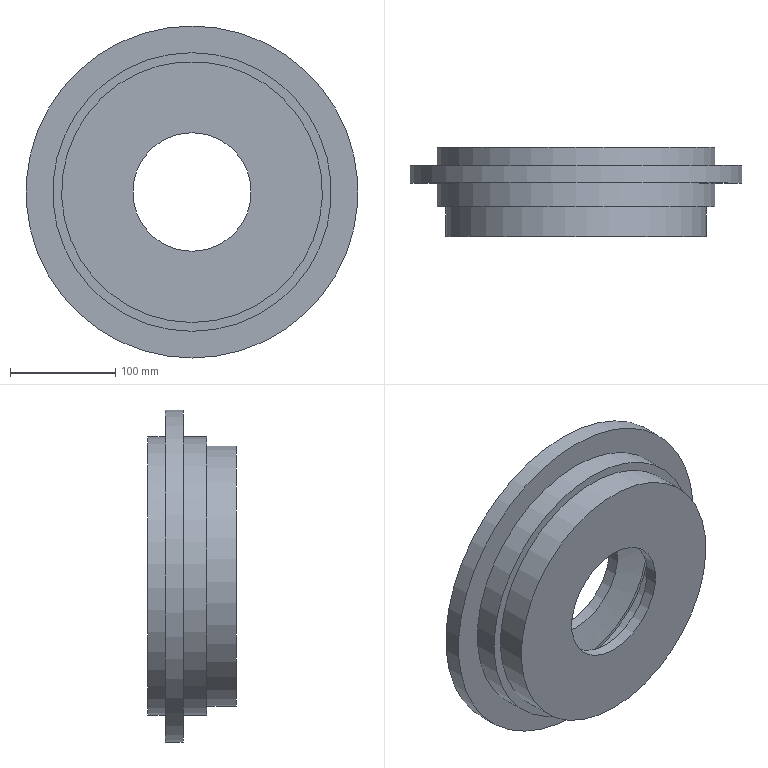Part | NX | features SIMPLE HOLE 4, CHAMFER 3, DATUM_CSYS 1, Delete Body 1, LINKED_BODY 1, SCALE 1, SKETCH 1, SWP104 1 | 1 solid | 18 faces | box 315 x 84.375 x 315 mm | volume 2887099 mm3 | plane 8 | cylinder 8 | cone 2 | commonest cylinder face diameters 112.5 x2 264.375 x2 185.625 x1 208.125 x1 247.5 x1 315 x1
STEP:
#1=CARTESIAN_POINT('',(-2029.479,-199.375,-310.332));
#2=VERTEX_POINT('',#1);
#3=CARTESIAN_POINT('',(-2029.479,-199.375,-366.582));
#4=DIRECTION('',(0.,1.,0.));
#5=DIRECTION('',(0.,0.,1.));
#6=AXIS2_PLACEMENT_3D('',#3,#4,#5);
#7=CIRCLE('',#6,56.25);
#8=EDGE_CURVE('',#2,#2,#7,.T.);
#9=ORIENTED_EDGE('',*,*,#8,.T.);
#10=EDGE_LOOP('',(#9));
#11=FACE_BOUND('',#10,.T.);
#12=CARTESIAN_POINT('',(-2029.479,-199.375,-490.332));
#13=VERTEX_POINT('',#12);
#14=CARTESIAN_POINT('',(-2029.479,-199.375,-366.582));
#15=DIRECTION('',(0.,-1.,0.));
#16=DIRECTION('',(0.,0.,-1.));
#17=AXIS2_PLACEMENT_3D('',#14,#15,#16);
#18=CIRCLE('',#17,123.75);
#19=EDGE_CURVE('',#13,#13,#18,.T.);
#20=ORIENTED_EDGE('',*,*,#19,.T.);
#21=EDGE_LOOP('',(#20));
#22=FACE_BOUND('',#21,.T.);
#23=CARTESIAN_POINT('',(-2029.479,-199.375,-366.582));
#24=DIRECTION('',(0.,-1.,0.));
#25=DIRECTION('',(0.,0.,-1.));
#26=AXIS2_PLACEMENT_3D('',#23,#24,#25);
#27=PLANE('',#26);
#28=ADVANCED_FACE('',(#11,#22),#27,.T.);
#29=CARTESIAN_POINT('',(-2029.479,-171.25,-490.332));
#30=VERTEX_POINT('',#29);
#31=CARTESIAN_POINT('',(-2029.479,-171.25,-366.582));
#32=DIRECTION('',(0.,-1.,0.));
#33=DIRECTION('',(0.,0.,-1.));
#34=AXIS2_PLACEMENT_3D('',#31,#32,#33);
#35=CIRCLE('',#34,123.75);
#36=EDGE_CURVE('',#30,#30,#35,.T.);
#37=ORIENTED_EDGE('',*,*,#36,.T.);
#38=EDGE_LOOP('',(#37));
#39=FACE_BOUND('',#38,.T.);
#40=ORIENTED_EDGE('',*,*,#19,.F.);
#41=EDGE_LOOP('',(#40));
#42=FACE_BOUND('',#41,.T.);
#43=CARTESIAN_POINT('',(-2029.479,-199.375,-366.582));
#44=DIRECTION('',(0.,-1.,0.));
#45=DIRECTION('',(0.,0.,-1.));
#46=AXIS2_PLACEMENT_3D('',#43,#44,#45);
#47=CYLINDRICAL_SURFACE('',#46,123.75);
#48=ADVANCED_FACE('',(#39,#42),#47,.T.);
#49=CARTESIAN_POINT('',(-2029.479,-171.25,-498.77));
#50=VERTEX_POINT('',#49);
#51=CARTESIAN_POINT('',(-2029.479,-171.25,-366.582));
#52=DIRECTION('',(0.,-1.,0.));
#53=DIRECTION('',(0.,0.,-1.));
#54=AXIS2_PLACEMENT_3D('',#51,#52,#53);
#55=CIRCLE('',#54,132.188);
#56=EDGE_CURVE('',#50,#50,#55,.T.);
#57=ORIENTED_EDGE('',*,*,#56,.T.);
#58=EDGE_LOOP('',(#57));
#59=FACE_BOUND('',#58,.T.);
#60=ORIENTED_EDGE('',*,*,#36,.F.);
#61=EDGE_LOOP('',(#60));
#62=FACE_BOUND('',#61,.T.);
#63=CARTESIAN_POINT('',(-2029.479,-171.25,-242.832));
#64=DIRECTION('',(0.,-1.,0.));
#65=DIRECTION('',(0.,0.,-1.));
#66=AXIS2_PLACEMENT_3D('',#63,#64,#65);
#67=PLANE('',#66);
#68=ADVANCED_FACE('',(#59,#62),#67,.T.);
#69=CARTESIAN_POINT('',(-2029.479,-148.75,-498.77));
#70=VERTEX_POINT('',#69);
#71=CARTESIAN_POINT('',(-2029.479,-148.75,-366.582));
#72=DIRECTION('',(0.,-1.,0.));
#73=DIRECTION('',(0.,0.,-1.));
#74=AXIS2_PLACEMENT_3D('',#71,#72,#73);
#75=CIRCLE('',#74,132.188);
#76=EDGE_CURVE('',#70,#70,#75,.T.);
#77=ORIENTED_EDGE('',*,*,#76,.T.);
#78=EDGE_LOOP('',(#77));
#79=FACE_BOUND('',#78,.T.);
#80=ORIENTED_EDGE('',*,*,#56,.F.);
#81=EDGE_LOOP('',(#80));
#82=FACE_BOUND('',#81,.T.);
#83=CARTESIAN_POINT('',(-2029.479,-199.375,-366.582));
#84=DIRECTION('',(0.,-1.,0.));
#85=DIRECTION('',(0.,0.,-1.));
#86=AXIS2_PLACEMENT_3D('',#83,#84,#85);
#87=CYLINDRICAL_SURFACE('',#86,132.188);
#88=ADVANCED_FACE('',(#79,#82),#87,.T.);
#89=CARTESIAN_POINT('',(-2029.479,-148.75,-524.082));
#90=VERTEX_POINT('',#89);
#91=CARTESIAN_POINT('',(-2029.479,-148.75,-366.582));
#92=DIRECTION('',(0.,-1.,0.));
#93=DIRECTION('',(0.,0.,-1.));
#94=AXIS2_PLACEMENT_3D('',#91,#92,#93);
#95=CIRCLE('',#94,157.5);
#96=EDGE_CURVE('',#90,#90,#95,.T.);
#97=ORIENTED_EDGE('',*,*,#96,.T.);
#98=EDGE_LOOP('',(#97));
#99=FACE_BOUND('',#98,.T.);
#100=ORIENTED_EDGE('',*,*,#76,.F.);
#101=EDGE_LOOP('',(#100));
#102=FACE_BOUND('',#101,.T.);
#103=CARTESIAN_POINT('',(-2029.479,-148.75,-234.395));
#104=DIRECTION('',(0.,-1.,0.));
#105=DIRECTION('',(0.,0.,-1.));
#106=AXIS2_PLACEMENT_3D('',#103,#104,#105);
#107=PLANE('',#106);
#108=ADVANCED_FACE('',(#99,#102),#107,.T.);
#109=CARTESIAN_POINT('',(-2029.479,-131.875,-524.082));
#110=VERTEX_POINT('',#109);
#111=CARTESIAN_POINT('',(-2029.479,-131.875,-366.582));
#112=DIRECTION('',(0.,-1.,0.));
#113=DIRECTION('',(0.,0.,-1.));
#114=AXIS2_PLACEMENT_3D('',#111,#112,#113);
#115=CIRCLE('',#114,157.5);
#116=EDGE_CURVE('',#110,#110,#115,.T.);
#117=ORIENTED_EDGE('',*,*,#116,.T.);
#118=EDGE_LOOP('',(#117));
#119=FACE_BOUND('',#118,.T.);
#120=ORIENTED_EDGE('',*,*,#96,.F.);
#121=EDGE_LOOP('',(#120));
#122=FACE_BOUND('',#121,.T.);
#123=CARTESIAN_POINT('',(-2029.479,-199.375,-366.582));
#124=DIRECTION('',(0.,-1.,0.));
#125=DIRECTION('',(0.,0.,-1.));
#126=AXIS2_PLACEMENT_3D('',#123,#124,#125);
#127=CYLINDRICAL_SURFACE('',#126,157.5);
#128=ADVANCED_FACE('',(#119,#122),#127,.T.);
#129=CARTESIAN_POINT('',(-2029.479,-131.875,-498.77));
#130=VERTEX_POINT('',#129);
#131=CARTESIAN_POINT('',(-2029.479,-131.875,-366.582));
#132=DIRECTION('',(0.,-1.,0.));
#133=DIRECTION('',(0.,0.,-1.));
#134=AXIS2_PLACEMENT_3D('',#131,#132,#133);
#135=CIRCLE('',#134,132.188);
#136=EDGE_CURVE('',#130,#130,#135,.T.);
#137=ORIENTED_EDGE('',*,*,#136,.T.);
#138=EDGE_LOOP('',(#137));
#139=FACE_BOUND('',#138,.T.);
#140=ORIENTED_EDGE('',*,*,#116,.F.);
#141=EDGE_LOOP('',(#140));
#142=FACE_BOUND('',#141,.T.);
#143=CARTESIAN_POINT('',(-2029.479,-131.875,-209.082));
#144=DIRECTION('',(0.,1.,0.));
#145=DIRECTION('',(0.,0.,1.));
#146=AXIS2_PLACEMENT_3D('',#143,#144,#145);
#147=PLANE('',#146);
#148=ADVANCED_FACE('',(#139,#142),#147,.T.);
#149=CARTESIAN_POINT('',(-2029.479,-115.,-498.77));
#150=VERTEX_POINT('',#149);
#151=CARTESIAN_POINT('',(-2029.479,-115.,-366.582));
#152=DIRECTION('',(0.,-1.,0.));
#153=DIRECTION('',(0.,0.,-1.));
#154=AXIS2_PLACEMENT_3D('',#151,#152,#153);
#155=CIRCLE('',#154,132.188);
#156=EDGE_CURVE('',#150,#150,#155,.T.);
#157=ORIENTED_EDGE('',*,*,#156,.T.);
#158=EDGE_LOOP('',(#157));
#159=FACE_BOUND('',#158,.T.);
#160=ORIENTED_EDGE('',*,*,#136,.F.);
#161=EDGE_LOOP('',(#160));
#162=FACE_BOUND('',#161,.T.);
#163=CARTESIAN_POINT('',(-2029.479,-199.375,-366.582));
#164=DIRECTION('',(0.,-1.,0.));
#165=DIRECTION('',(0.,0.,-1.));
#166=AXIS2_PLACEMENT_3D('',#163,#164,#165);
#167=CYLINDRICAL_SURFACE('',#166,132.188);
#168=ADVANCED_FACE('',(#159,#162),#167,.T.);
#169=CARTESIAN_POINT('',(-2029.479,-115.,-470.645));
#170=VERTEX_POINT('',#169);
#171=CARTESIAN_POINT('',(-2029.479,-115.,-366.582));
#172=DIRECTION('',(0.,-1.,0.));
#173=DIRECTION('',(0.,0.,-1.));
#174=AXIS2_PLACEMENT_3D('',#171,#172,#173);
#175=CIRCLE('',#174,104.062);
#176=EDGE_CURVE('',#170,#170,#175,.T.);
#177=ORIENTED_EDGE('',*,*,#176,.T.);
#178=EDGE_LOOP('',(#177));
#179=FACE_BOUND('',#178,.T.);
#180=ORIENTED_EDGE('',*,*,#156,.F.);
#181=EDGE_LOOP('',(#180));
#182=FACE_BOUND('',#181,.T.);
#183=CARTESIAN_POINT('',(-2029.479,-115.,-234.395));
#184=DIRECTION('',(0.,1.,0.));
#185=DIRECTION('',(0.,0.,1.));
#186=AXIS2_PLACEMENT_3D('',#183,#184,#185);
#187=PLANE('',#186);
#188=ADVANCED_FACE('',(#179,#182),#187,.T.);
#189=CARTESIAN_POINT('',(-2029.479,-188.125,-422.832));
#190=VERTEX_POINT('',#189);
#191=CARTESIAN_POINT('',(-2029.479,-188.125,-366.582));
#192=DIRECTION('',(0.,-1.,0.));
#193=DIRECTION('',(0.,0.,-1.));
#194=AXIS2_PLACEMENT_3D('',#191,#192,#193);
#195=CIRCLE('',#194,56.25);
#196=EDGE_CURVE('',#190,#190,#195,.F.);
#197=ORIENTED_EDGE('',*,*,#196,.T.);
#198=EDGE_LOOP('',(#197));
#199=FACE_BOUND('',#198,.T.);
#200=ORIENTED_EDGE('',*,*,#8,.F.);
#201=EDGE_LOOP('',(#200));
#202=FACE_BOUND('',#201,.T.);
#203=CARTESIAN_POINT('',(-2029.479,-199.375,-366.582));
#204=DIRECTION('',(0.,1.,0.));
#205=DIRECTION('',(0.,0.,1.));
#206=AXIS2_PLACEMENT_3D('',#203,#204,#205);
#207=CYLINDRICAL_SURFACE('',#206,56.25);
#208=ADVANCED_FACE('',(#199,#202),#207,.F.);
#209=CARTESIAN_POINT('',(-2029.479,-137.5,-422.832));
#210=VERTEX_POINT('',#209);
#211=CARTESIAN_POINT('',(-2029.479,-137.5,-366.582));
#212=DIRECTION('',(0.,-1.,0.));
#213=DIRECTION('',(0.,0.,-1.));
#214=AXIS2_PLACEMENT_3D('',#211,#212,#213);
#215=CIRCLE('',#214,56.25);
#216=EDGE_CURVE('',#210,#210,#215,.T.);
#217=ORIENTED_EDGE('',*,*,#216,.T.);
#218=EDGE_LOOP('',(#217));
#219=FACE_BOUND('',#218,.T.);
#220=CARTESIAN_POINT('',(-2029.479,-137.5,-470.645));
#221=VERTEX_POINT('',#220);
#222=CARTESIAN_POINT('',(-2029.479,-137.5,-366.582));
#223=DIRECTION('',(0.,-1.,0.));
#224=DIRECTION('',(0.,0.,-1.));
#225=AXIS2_PLACEMENT_3D('',#222,#223,#224);
#226=CIRCLE('',#225,104.062);
#227=EDGE_CURVE('',#221,#221,#226,.F.);
#228=ORIENTED_EDGE('',*,*,#227,.T.);
#229=EDGE_LOOP('',(#228));
#230=FACE_BOUND('',#229,.T.);
#231=CARTESIAN_POINT('',(-2029.479,-137.5,-366.582));
#232=DIRECTION('',(0.,-1.,0.));
#233=DIRECTION('',(0.,0.,-1.));
#234=AXIS2_PLACEMENT_3D('',#231,#232,#233);
#235=PLANE('',#234);
#236=ADVANCED_FACE('',(#219,#230),#235,.F.);
#237=ORIENTED_EDGE('',*,*,#227,.F.);
#238=EDGE_LOOP('',(#237));
#239=FACE_BOUND('',#238,.T.);
#240=ORIENTED_EDGE('',*,*,#176,.F.);
#241=EDGE_LOOP('',(#240));
#242=FACE_BOUND('',#241,.T.);
#243=CARTESIAN_POINT('',(-2029.479,-115.,-366.582));
#244=DIRECTION('',(0.,-1.,0.));
#245=DIRECTION('',(0.,0.,-1.));
#246=AXIS2_PLACEMENT_3D('',#243,#244,#245);
#247=CYLINDRICAL_SURFACE('',#246,104.062);
#248=ADVANCED_FACE('',(#239,#242),#247,.F.);
#249=CARTESIAN_POINT('',(-2029.479,-148.75,-310.332));
#250=VERTEX_POINT('',#249);
#251=CARTESIAN_POINT('',(-2029.479,-148.75,-366.582));
#252=DIRECTION('',(0.,1.,0.));
#253=DIRECTION('',(0.,0.,1.));
#254=AXIS2_PLACEMENT_3D('',#251,#252,#253);
#255=CIRCLE('',#254,56.25);
#256=EDGE_CURVE('',#250,#250,#255,.F.);
#257=ORIENTED_EDGE('',*,*,#256,.T.);
#258=EDGE_LOOP('',(#257));
#259=FACE_BOUND('',#258,.T.);
#260=ORIENTED_EDGE('',*,*,#216,.F.);
#261=EDGE_LOOP('',(#260));
#262=FACE_BOUND('',#261,.T.);
#263=CARTESIAN_POINT('',(-2029.479,-137.5,-366.582));
#264=DIRECTION('',(0.,-1.,0.));
#265=DIRECTION('',(0.,0.,-1.));
#266=AXIS2_PLACEMENT_3D('',#263,#264,#265);
#267=CYLINDRICAL_SURFACE('',#266,56.25);
#268=ADVANCED_FACE('',(#259,#262),#267,.F.);
#269=CARTESIAN_POINT('',(-2029.479,-182.5,-456.582));
#270=VERTEX_POINT('',#269);
#271=CARTESIAN_POINT('',(-2029.479,-182.5,-366.582));
#272=DIRECTION('',(0.,-1.,0.));
#273=DIRECTION('',(0.,0.,-1.));
#274=AXIS2_PLACEMENT_3D('',#271,#272,#273);
#275=CIRCLE('',#274,90.);
#276=EDGE_CURVE('',#270,#270,#275,.T.);
#277=ORIENTED_EDGE('',*,*,#276,.T.);
#278=EDGE_LOOP('',(#277));
#279=FACE_BOUND('',#278,.T.);
#280=CARTESIAN_POINT('',(-2029.479,-182.5,-459.395));
#281=VERTEX_POINT('',#280);
#282=CARTESIAN_POINT('',(-2029.479,-182.5,-366.582));
#283=DIRECTION('',(0.,-1.,0.));
#284=DIRECTION('',(0.,0.,-1.));
#285=AXIS2_PLACEMENT_3D('',#282,#283,#284);
#286=CIRCLE('',#285,92.812);
#287=EDGE_CURVE('',#281,#281,#286,.F.);
#288=ORIENTED_EDGE('',*,*,#287,.T.);
#289=EDGE_LOOP('',(#288));
#290=FACE_BOUND('',#289,.T.);
#291=CARTESIAN_POINT('',(-2029.479,-182.5,-366.582));
#292=DIRECTION('',(0.,-1.,0.));
#293=DIRECTION('',(0.,0.,-1.));
#294=AXIS2_PLACEMENT_3D('',#291,#292,#293);
#295=PLANE('',#294);
#296=ADVANCED_FACE('',(#279,#290),#295,.F.);
#297=CARTESIAN_POINT('',(-2029.479,-154.375,-276.582));
#298=VERTEX_POINT('',#297);
#299=CARTESIAN_POINT('',(-2029.479,-154.375,-366.582));
#300=DIRECTION('',(0.,1.,0.));
#301=DIRECTION('',(0.,0.,1.));
#302=AXIS2_PLACEMENT_3D('',#299,#300,#301);
#303=CIRCLE('',#302,90.);
#304=EDGE_CURVE('',#298,#298,#303,.T.);
#305=ORIENTED_EDGE('',*,*,#304,.T.);
#306=EDGE_LOOP('',(#305));
#307=FACE_BOUND('',#306,.T.);
#308=CARTESIAN_POINT('',(-2029.479,-154.375,-459.395));
#309=VERTEX_POINT('',#308);
#310=CARTESIAN_POINT('',(-2029.479,-154.375,-366.582));
#311=DIRECTION('',(0.,-1.,0.));
#312=DIRECTION('',(0.,0.,-1.));
#313=AXIS2_PLACEMENT_3D('',#310,#311,#312);
#314=CIRCLE('',#313,92.812);
#315=EDGE_CURVE('',#309,#309,#314,.F.);
#316=ORIENTED_EDGE('',*,*,#315,.F.);
#317=EDGE_LOOP('',(#316));
#318=FACE_BOUND('',#317,.T.);
#319=CARTESIAN_POINT('',(-2029.479,-154.375,-366.582));
#320=DIRECTION('',(0.,1.,0.));
#321=DIRECTION('',(0.,0.,1.));
#322=AXIS2_PLACEMENT_3D('',#319,#320,#321);
#323=PLANE('',#322);
#324=ADVANCED_FACE('',(#307,#318),#323,.F.);
#325=ORIENTED_EDGE('',*,*,#287,.F.);
#326=EDGE_LOOP('',(#325));
#327=FACE_BOUND('',#326,.T.);
#328=ORIENTED_EDGE('',*,*,#315,.T.);
#329=EDGE_LOOP('',(#328));
#330=FACE_BOUND('',#329,.T.);
#331=CARTESIAN_POINT('',(-2029.479,-154.375,-366.582));
#332=DIRECTION('',(0.,-1.,0.));
#333=DIRECTION('',(0.,0.,-1.));
#334=AXIS2_PLACEMENT_3D('',#331,#332,#333);
#335=CYLINDRICAL_SURFACE('',#334,92.812);
#336=ADVANCED_FACE('',(#327,#330),#335,.F.);
#337=ORIENTED_EDGE('',*,*,#276,.F.);
#338=EDGE_LOOP('',(#337));
#339=FACE_BOUND('',#338,.T.);
#340=ORIENTED_EDGE('',*,*,#196,.F.);
#341=EDGE_LOOP('',(#340));
#342=FACE_BOUND('',#341,.T.);
#343=CARTESIAN_POINT('',(-2029.479,-188.125,-366.582));
#344=DIRECTION('',(0.,1.,0.));
#345=DIRECTION('',(0.,0.,1.));
#346=AXIS2_PLACEMENT_3D('',#343,#344,#345);
#347=CONICAL_SURFACE('',#346,56.25,1.406);
#348=ADVANCED_FACE('',(#339,#342),#347,.F.);
#349=ORIENTED_EDGE('',*,*,#304,.F.);
#350=EDGE_LOOP('',(#349));
#351=FACE_BOUND('',#350,.T.);
#352=ORIENTED_EDGE('',*,*,#256,.F.);
#353=EDGE_LOOP('',(#352));
#354=FACE_BOUND('',#353,.T.);
#355=CARTESIAN_POINT('',(-2029.479,-148.75,-366.582));
#356=DIRECTION('',(0.,-1.,0.));
#357=DIRECTION('',(0.,0.,-1.));
#358=AXIS2_PLACEMENT_3D('',#355,#356,#357);
#359=CONICAL_SURFACE('',#358,56.25,1.406);
#360=ADVANCED_FACE('',(#351,#354),#359,.F.);
#361=CLOSED_SHELL('',(#28,#48,#68,#88,#108,#128,#148,#168,#188,#208,#236,#248,#268,#296,#324,#336,#348,#360));
#362=MANIFOLD_SOLID_BREP('',#361);
#363=(LENGTH_UNIT()NAMED_UNIT(*)SI_UNIT(.MILLI.,.METRE.));
#364=UNCERTAINTY_MEASURE_WITH_UNIT(LENGTH_MEASURE(0.00001),#363,'','');
#365=(NAMED_UNIT(*)PLANE_ANGLE_UNIT()SI_UNIT($,.RADIAN.));
#366=(NAMED_UNIT(*)SI_UNIT($,.STERADIAN.)SOLID_ANGLE_UNIT());
#367=(GEOMETRIC_REPRESENTATION_CONTEXT(3)GLOBAL_UNCERTAINTY_ASSIGNED_CONTEXT((#364))GLOBAL_UNIT_ASSIGNED_CONTEXT((#363,#365,#366))REPRESENTATION_CONTEXT('',''));
#368=ADVANCED_BREP_SHAPE_REPRESENTATION('',(#362),#367);